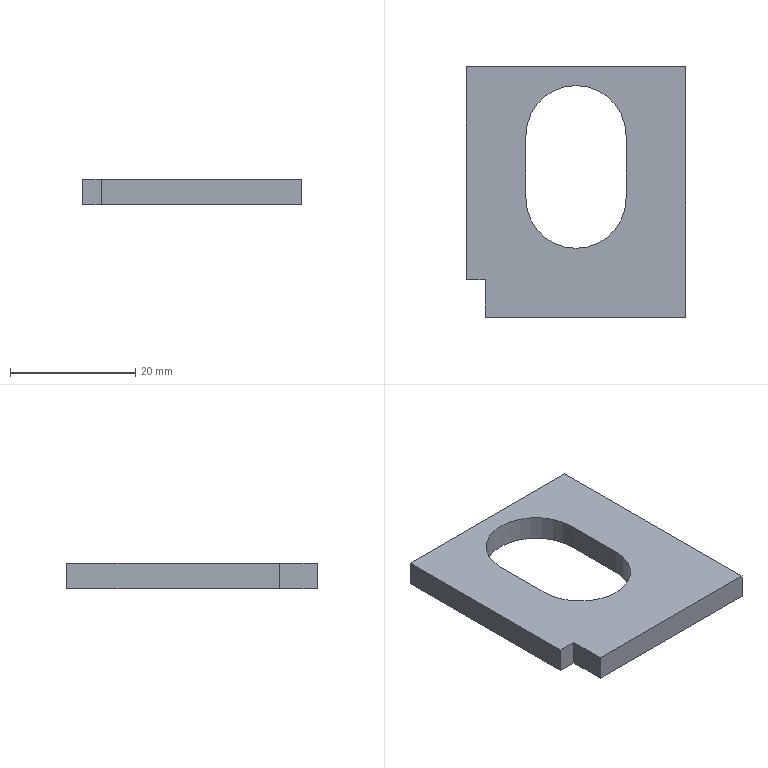Part | SolidWorks | features Extrusion 1 | 1 solid | 12 faces | box 35 x 40 x 4 mm | volume 4084 mm3 | plane 10 | cylinder 2 | commonest cylinder face diameters 16 x2
STEP:
#1=CARTESIAN_POINT('',(35.,0.,4.));
#2=VERTEX_POINT('',#1);
#3=CARTESIAN_POINT('',(35.,40.,4.));
#4=VERTEX_POINT('',#3);
#5=CARTESIAN_POINT('',(35.,0.,4.));
#6=DIRECTION('',(0.,1.,0.));
#7=VECTOR('',#6,1000.);
#8=LINE('',#5,#7);
#9=EDGE_CURVE('',#2,#4,#8,.T.);
#10=ORIENTED_EDGE('',*,*,#9,.T.);
#11=CARTESIAN_POINT('',(0.,40.,4.));
#12=VERTEX_POINT('',#11);
#13=CARTESIAN_POINT('',(0.,40.,4.));
#14=DIRECTION('',(-1.,0.,0.));
#15=VECTOR('',#14,1000.);
#16=LINE('',#13,#15);
#17=EDGE_CURVE('',#4,#12,#16,.T.);
#18=ORIENTED_EDGE('',*,*,#17,.T.);
#19=CARTESIAN_POINT('',(0.,5.998,4.));
#20=VERTEX_POINT('',#19);
#21=CARTESIAN_POINT('',(0.,5.998,4.));
#22=DIRECTION('',(0.,-1.,0.));
#23=VECTOR('',#22,1000.);
#24=LINE('',#21,#23);
#25=EDGE_CURVE('',#12,#20,#24,.T.);
#26=ORIENTED_EDGE('',*,*,#25,.T.);
#27=CARTESIAN_POINT('',(3.,5.998,4.));
#28=VERTEX_POINT('',#27);
#29=CARTESIAN_POINT('',(0.,5.998,4.));
#30=DIRECTION('',(1.,0.,0.));
#31=VECTOR('',#30,1000.);
#32=LINE('',#29,#31);
#33=EDGE_CURVE('',#20,#28,#32,.T.);
#34=ORIENTED_EDGE('',*,*,#33,.T.);
#35=CARTESIAN_POINT('',(3.,0.,4.));
#36=VERTEX_POINT('',#35);
#37=CARTESIAN_POINT('',(3.,5.998,4.));
#38=DIRECTION('',(0.,-1.,0.));
#39=VECTOR('',#38,1000.);
#40=LINE('',#37,#39);
#41=EDGE_CURVE('',#28,#36,#40,.T.);
#42=ORIENTED_EDGE('',*,*,#41,.T.);
#43=CARTESIAN_POINT('',(3.,0.,4.));
#44=DIRECTION('',(1.,0.,0.));
#45=VECTOR('',#44,1000.);
#46=LINE('',#43,#45);
#47=EDGE_CURVE('',#36,#2,#46,.T.);
#48=ORIENTED_EDGE('',*,*,#47,.T.);
#49=EDGE_LOOP('',(#10,#18,#26,#34,#42,#48));
#50=FACE_OUTER_BOUND('',#49,.T.);
#51=CARTESIAN_POINT('',(25.5,29.,4.));
#52=VERTEX_POINT('',#51);
#53=CARTESIAN_POINT('',(9.5,29.,4.));
#54=VERTEX_POINT('',#53);
#55=CARTESIAN_POINT('',(17.5,29.,4.));
#56=DIRECTION('',(0.,0.,1.));
#57=DIRECTION('',(1.,0.,0.));
#58=AXIS2_PLACEMENT_3D('',#55,#56,#57);
#59=CIRCLE('',#58,8.);
#60=EDGE_CURVE('',#52,#54,#59,.T.);
#61=ORIENTED_EDGE('',*,*,#60,.F.);
#62=CARTESIAN_POINT('',(25.5,19.,4.));
#63=VERTEX_POINT('',#62);
#64=CARTESIAN_POINT('',(25.5,29.,4.));
#65=DIRECTION('',(0.,1.,0.));
#66=VECTOR('',#65,1000.);
#67=LINE('',#64,#66);
#68=EDGE_CURVE('',#63,#52,#67,.T.);
#69=ORIENTED_EDGE('',*,*,#68,.F.);
#70=CARTESIAN_POINT('',(9.5,19.,4.));
#71=VERTEX_POINT('',#70);
#72=CARTESIAN_POINT('',(17.5,19.,4.));
#73=DIRECTION('',(0.,0.,1.));
#74=DIRECTION('',(1.,0.,0.));
#75=AXIS2_PLACEMENT_3D('',#72,#73,#74);
#76=CIRCLE('',#75,8.);
#77=EDGE_CURVE('',#71,#63,#76,.T.);
#78=ORIENTED_EDGE('',*,*,#77,.F.);
#79=CARTESIAN_POINT('',(9.5,29.,4.));
#80=DIRECTION('',(0.,-1.,0.));
#81=VECTOR('',#80,1000.);
#82=LINE('',#79,#81);
#83=EDGE_CURVE('',#54,#71,#82,.T.);
#84=ORIENTED_EDGE('',*,*,#83,.F.);
#85=EDGE_LOOP('',(#61,#69,#78,#84));
#86=FACE_BOUND('',#85,.T.);
#87=CARTESIAN_POINT('',(0.,0.,4.));
#88=DIRECTION('',(0.,0.,-1.));
#89=DIRECTION('',(-1.,0.,0.));
#90=AXIS2_PLACEMENT_3D('',#87,#88,#89);
#91=PLANE('',#90);
#92=ADVANCED_FACE('',(#50,#86),#91,.F.);
#93=CARTESIAN_POINT('',(35.,0.,0.));
#94=VERTEX_POINT('',#93);
#95=CARTESIAN_POINT('',(35.,40.,0.));
#96=VERTEX_POINT('',#95);
#97=CARTESIAN_POINT('',(35.,0.,0.));
#98=DIRECTION('',(0.,1.,0.));
#99=VECTOR('',#98,1000.);
#100=LINE('',#97,#99);
#101=EDGE_CURVE('',#94,#96,#100,.T.);
#102=ORIENTED_EDGE('',*,*,#101,.F.);
#103=CARTESIAN_POINT('',(3.,0.,0.));
#104=VERTEX_POINT('',#103);
#105=CARTESIAN_POINT('',(3.,0.,0.));
#106=DIRECTION('',(1.,0.,0.));
#107=VECTOR('',#106,1000.);
#108=LINE('',#105,#107);
#109=EDGE_CURVE('',#104,#94,#108,.T.);
#110=ORIENTED_EDGE('',*,*,#109,.F.);
#111=CARTESIAN_POINT('',(3.,5.998,0.));
#112=VERTEX_POINT('',#111);
#113=CARTESIAN_POINT('',(3.,5.998,0.));
#114=DIRECTION('',(0.,-1.,0.));
#115=VECTOR('',#114,1000.);
#116=LINE('',#113,#115);
#117=EDGE_CURVE('',#112,#104,#116,.T.);
#118=ORIENTED_EDGE('',*,*,#117,.F.);
#119=CARTESIAN_POINT('',(0.,5.998,0.));
#120=VERTEX_POINT('',#119);
#121=CARTESIAN_POINT('',(0.,5.998,0.));
#122=DIRECTION('',(1.,0.,0.));
#123=VECTOR('',#122,1000.);
#124=LINE('',#121,#123);
#125=EDGE_CURVE('',#120,#112,#124,.T.);
#126=ORIENTED_EDGE('',*,*,#125,.F.);
#127=CARTESIAN_POINT('',(0.,40.,0.));
#128=VERTEX_POINT('',#127);
#129=CARTESIAN_POINT('',(0.,5.998,0.));
#130=DIRECTION('',(0.,-1.,0.));
#131=VECTOR('',#130,1000.);
#132=LINE('',#129,#131);
#133=EDGE_CURVE('',#128,#120,#132,.T.);
#134=ORIENTED_EDGE('',*,*,#133,.F.);
#135=CARTESIAN_POINT('',(0.,40.,0.));
#136=DIRECTION('',(-1.,0.,0.));
#137=VECTOR('',#136,1000.);
#138=LINE('',#135,#137);
#139=EDGE_CURVE('',#96,#128,#138,.T.);
#140=ORIENTED_EDGE('',*,*,#139,.F.);
#141=EDGE_LOOP('',(#102,#110,#118,#126,#134,#140));
#142=FACE_OUTER_BOUND('',#141,.T.);
#143=CARTESIAN_POINT('',(25.5,19.,0.));
#144=VERTEX_POINT('',#143);
#145=CARTESIAN_POINT('',(25.5,29.,0.));
#146=VERTEX_POINT('',#145);
#147=CARTESIAN_POINT('',(25.5,29.,0.));
#148=DIRECTION('',(0.,1.,0.));
#149=VECTOR('',#148,1000.);
#150=LINE('',#147,#149);
#151=EDGE_CURVE('',#144,#146,#150,.T.);
#152=ORIENTED_EDGE('',*,*,#151,.T.);
#153=CARTESIAN_POINT('',(9.5,29.,0.));
#154=VERTEX_POINT('',#153);
#155=CARTESIAN_POINT('',(17.5,29.,0.));
#156=DIRECTION('',(0.,0.,1.));
#157=DIRECTION('',(1.,0.,0.));
#158=AXIS2_PLACEMENT_3D('',#155,#156,#157);
#159=CIRCLE('',#158,8.);
#160=EDGE_CURVE('',#146,#154,#159,.T.);
#161=ORIENTED_EDGE('',*,*,#160,.T.);
#162=CARTESIAN_POINT('',(9.5,19.,0.));
#163=VERTEX_POINT('',#162);
#164=CARTESIAN_POINT('',(9.5,29.,0.));
#165=DIRECTION('',(0.,-1.,0.));
#166=VECTOR('',#165,1000.);
#167=LINE('',#164,#166);
#168=EDGE_CURVE('',#154,#163,#167,.T.);
#169=ORIENTED_EDGE('',*,*,#168,.T.);
#170=CARTESIAN_POINT('',(17.5,19.,0.));
#171=DIRECTION('',(0.,0.,1.));
#172=DIRECTION('',(1.,0.,0.));
#173=AXIS2_PLACEMENT_3D('',#170,#171,#172);
#174=CIRCLE('',#173,8.);
#175=EDGE_CURVE('',#163,#144,#174,.T.);
#176=ORIENTED_EDGE('',*,*,#175,.T.);
#177=EDGE_LOOP('',(#152,#161,#169,#176));
#178=FACE_BOUND('',#177,.T.);
#179=CARTESIAN_POINT('',(0.,0.,0.));
#180=DIRECTION('',(0.,0.,-1.));
#181=DIRECTION('',(-1.,0.,0.));
#182=AXIS2_PLACEMENT_3D('',#179,#180,#181);
#183=PLANE('',#182);
#184=ADVANCED_FACE('',(#142,#178),#183,.T.);
#185=ORIENTED_EDGE('',*,*,#101,.T.);
#186=CARTESIAN_POINT('',(35.,40.,4.));
#187=DIRECTION('',(0.,0.,-1.));
#188=VECTOR('',#187,1000.);
#189=LINE('',#186,#188);
#190=EDGE_CURVE('',#4,#96,#189,.T.);
#191=ORIENTED_EDGE('',*,*,#190,.F.);
#192=ORIENTED_EDGE('',*,*,#9,.F.);
#193=CARTESIAN_POINT('',(35.,0.,4.));
#194=DIRECTION('',(0.,0.,-1.));
#195=VECTOR('',#194,1000.);
#196=LINE('',#193,#195);
#197=EDGE_CURVE('',#2,#94,#196,.T.);
#198=ORIENTED_EDGE('',*,*,#197,.T.);
#199=EDGE_LOOP('',(#185,#191,#192,#198));
#200=FACE_OUTER_BOUND('',#199,.T.);
#201=CARTESIAN_POINT('',(35.,0.,4.));
#202=DIRECTION('',(-1.,0.,0.));
#203=DIRECTION('',(0.,0.,1.));
#204=AXIS2_PLACEMENT_3D('',#201,#202,#203);
#205=PLANE('',#204);
#206=ADVANCED_FACE('',(#200),#205,.F.);
#207=ORIENTED_EDGE('',*,*,#139,.T.);
#208=CARTESIAN_POINT('',(0.,40.,4.));
#209=DIRECTION('',(0.,0.,-1.));
#210=VECTOR('',#209,1000.);
#211=LINE('',#208,#210);
#212=EDGE_CURVE('',#12,#128,#211,.T.);
#213=ORIENTED_EDGE('',*,*,#212,.F.);
#214=ORIENTED_EDGE('',*,*,#17,.F.);
#215=ORIENTED_EDGE('',*,*,#190,.T.);
#216=EDGE_LOOP('',(#207,#213,#214,#215));
#217=FACE_OUTER_BOUND('',#216,.T.);
#218=CARTESIAN_POINT('',(0.,40.,4.));
#219=DIRECTION('',(0.,-1.,0.));
#220=DIRECTION('',(0.,0.,-1.));
#221=AXIS2_PLACEMENT_3D('',#218,#219,#220);
#222=PLANE('',#221);
#223=ADVANCED_FACE('',(#217),#222,.F.);
#224=ORIENTED_EDGE('',*,*,#133,.T.);
#225=CARTESIAN_POINT('',(0.,5.998,4.));
#226=DIRECTION('',(0.,0.,-1.));
#227=VECTOR('',#226,1000.);
#228=LINE('',#225,#227);
#229=EDGE_CURVE('',#20,#120,#228,.T.);
#230=ORIENTED_EDGE('',*,*,#229,.F.);
#231=ORIENTED_EDGE('',*,*,#25,.F.);
#232=ORIENTED_EDGE('',*,*,#212,.T.);
#233=EDGE_LOOP('',(#224,#230,#231,#232));
#234=FACE_OUTER_BOUND('',#233,.T.);
#235=CARTESIAN_POINT('',(0.,5.998,4.));
#236=DIRECTION('',(1.,0.,0.));
#237=DIRECTION('',(0.,0.,-1.));
#238=AXIS2_PLACEMENT_3D('',#235,#236,#237);
#239=PLANE('',#238);
#240=ADVANCED_FACE('',(#234),#239,.F.);
#241=ORIENTED_EDGE('',*,*,#125,.T.);
#242=CARTESIAN_POINT('',(3.,5.998,4.));
#243=DIRECTION('',(0.,0.,-1.));
#244=VECTOR('',#243,1000.);
#245=LINE('',#242,#244);
#246=EDGE_CURVE('',#28,#112,#245,.T.);
#247=ORIENTED_EDGE('',*,*,#246,.F.);
#248=ORIENTED_EDGE('',*,*,#33,.F.);
#249=ORIENTED_EDGE('',*,*,#229,.T.);
#250=EDGE_LOOP('',(#241,#247,#248,#249));
#251=FACE_OUTER_BOUND('',#250,.T.);
#252=CARTESIAN_POINT('',(0.,5.998,4.));
#253=DIRECTION('',(0.,1.,0.));
#254=DIRECTION('',(0.,0.,1.));
#255=AXIS2_PLACEMENT_3D('',#252,#253,#254);
#256=PLANE('',#255);
#257=ADVANCED_FACE('',(#251),#256,.F.);
#258=ORIENTED_EDGE('',*,*,#117,.T.);
#259=CARTESIAN_POINT('',(3.,0.,4.));
#260=DIRECTION('',(0.,0.,-1.));
#261=VECTOR('',#260,1000.);
#262=LINE('',#259,#261);
#263=EDGE_CURVE('',#36,#104,#262,.T.);
#264=ORIENTED_EDGE('',*,*,#263,.F.);
#265=ORIENTED_EDGE('',*,*,#41,.F.);
#266=ORIENTED_EDGE('',*,*,#246,.T.);
#267=EDGE_LOOP('',(#258,#264,#265,#266));
#268=FACE_OUTER_BOUND('',#267,.T.);
#269=CARTESIAN_POINT('',(3.,5.998,4.));
#270=DIRECTION('',(1.,0.,0.));
#271=DIRECTION('',(0.,0.,-1.));
#272=AXIS2_PLACEMENT_3D('',#269,#270,#271);
#273=PLANE('',#272);
#274=ADVANCED_FACE('',(#268),#273,.F.);
#275=ORIENTED_EDGE('',*,*,#109,.T.);
#276=ORIENTED_EDGE('',*,*,#197,.F.);
#277=ORIENTED_EDGE('',*,*,#47,.F.);
#278=ORIENTED_EDGE('',*,*,#263,.T.);
#279=EDGE_LOOP('',(#275,#276,#277,#278));
#280=FACE_OUTER_BOUND('',#279,.T.);
#281=CARTESIAN_POINT('',(3.,0.,4.));
#282=DIRECTION('',(0.,1.,0.));
#283=DIRECTION('',(0.,0.,1.));
#284=AXIS2_PLACEMENT_3D('',#281,#282,#283);
#285=PLANE('',#284);
#286=ADVANCED_FACE('',(#280),#285,.F.);
#287=ORIENTED_EDGE('',*,*,#160,.F.);
#288=CARTESIAN_POINT('',(25.5,29.,4.));
#289=DIRECTION('',(0.,0.,-1.));
#290=VECTOR('',#289,1000.);
#291=LINE('',#288,#290);
#292=EDGE_CURVE('',#52,#146,#291,.T.);
#293=ORIENTED_EDGE('',*,*,#292,.F.);
#294=ORIENTED_EDGE('',*,*,#60,.T.);
#295=CARTESIAN_POINT('',(9.5,29.,4.));
#296=DIRECTION('',(0.,0.,-1.));
#297=VECTOR('',#296,1000.);
#298=LINE('',#295,#297);
#299=EDGE_CURVE('',#54,#154,#298,.T.);
#300=ORIENTED_EDGE('',*,*,#299,.T.);
#301=EDGE_LOOP('',(#287,#293,#294,#300));
#302=FACE_OUTER_BOUND('',#301,.T.);
#303=CARTESIAN_POINT('',(17.5,29.,4.));
#304=DIRECTION('',(0.,0.,-1.));
#305=DIRECTION('',(-1.,0.,0.));
#306=AXIS2_PLACEMENT_3D('',#303,#304,#305);
#307=CYLINDRICAL_SURFACE('',#306,8.);
#308=ADVANCED_FACE('',(#302),#307,.F.);
#309=ORIENTED_EDGE('',*,*,#168,.F.);
#310=ORIENTED_EDGE('',*,*,#299,.F.);
#311=ORIENTED_EDGE('',*,*,#83,.T.);
#312=CARTESIAN_POINT('',(9.5,19.,4.));
#313=DIRECTION('',(0.,0.,-1.));
#314=VECTOR('',#313,1000.);
#315=LINE('',#312,#314);
#316=EDGE_CURVE('',#71,#163,#315,.T.);
#317=ORIENTED_EDGE('',*,*,#316,.T.);
#318=EDGE_LOOP('',(#309,#310,#311,#317));
#319=FACE_OUTER_BOUND('',#318,.T.);
#320=CARTESIAN_POINT('',(9.5,29.,4.));
#321=DIRECTION('',(1.,0.,0.));
#322=DIRECTION('',(0.,0.,-1.));
#323=AXIS2_PLACEMENT_3D('',#320,#321,#322);
#324=PLANE('',#323);
#325=ADVANCED_FACE('',(#319),#324,.T.);
#326=ORIENTED_EDGE('',*,*,#175,.F.);
#327=ORIENTED_EDGE('',*,*,#316,.F.);
#328=ORIENTED_EDGE('',*,*,#77,.T.);
#329=CARTESIAN_POINT('',(25.5,19.,4.));
#330=DIRECTION('',(0.,0.,-1.));
#331=VECTOR('',#330,1000.);
#332=LINE('',#329,#331);
#333=EDGE_CURVE('',#63,#144,#332,.T.);
#334=ORIENTED_EDGE('',*,*,#333,.T.);
#335=EDGE_LOOP('',(#326,#327,#328,#334));
#336=FACE_OUTER_BOUND('',#335,.T.);
#337=CARTESIAN_POINT('',(17.5,19.,4.));
#338=DIRECTION('',(0.,0.,-1.));
#339=DIRECTION('',(-1.,0.,0.));
#340=AXIS2_PLACEMENT_3D('',#337,#338,#339);
#341=CYLINDRICAL_SURFACE('',#340,8.);
#342=ADVANCED_FACE('',(#336),#341,.F.);
#343=ORIENTED_EDGE('',*,*,#151,.F.);
#344=ORIENTED_EDGE('',*,*,#333,.F.);
#345=ORIENTED_EDGE('',*,*,#68,.T.);
#346=ORIENTED_EDGE('',*,*,#292,.T.);
#347=EDGE_LOOP('',(#343,#344,#345,#346));
#348=FACE_OUTER_BOUND('',#347,.T.);
#349=CARTESIAN_POINT('',(25.5,29.,4.));
#350=DIRECTION('',(-1.,0.,0.));
#351=DIRECTION('',(0.,0.,1.));
#352=AXIS2_PLACEMENT_3D('',#349,#350,#351);
#353=PLANE('',#352);
#354=ADVANCED_FACE('',(#348),#353,.T.);
#355=CLOSED_SHELL('',(#92,#184,#206,#223,#240,#257,#274,#286,#308,#325,#342,#354));
#356=MANIFOLD_SOLID_BREP('',#355);
#357=CARTESIAN_POINT('',(0.,0.,0.));
#358=DIRECTION('',(0.,0.,1.));
#359=DIRECTION('',(1.,0.,0.));
#360=AXIS2_PLACEMENT_3D('',#357,#358,#359);
#361=(LENGTH_UNIT()NAMED_UNIT(*)SI_UNIT(.MILLI.,.METRE.));
#362=UNCERTAINTY_MEASURE_WITH_UNIT(LENGTH_MEASURE(0.00001),#361,'','');
#363=(NAMED_UNIT(*)PLANE_ANGLE_UNIT()SI_UNIT($,.RADIAN.));
#364=(NAMED_UNIT(*)SI_UNIT($,.STERADIAN.)SOLID_ANGLE_UNIT());
#365=(GEOMETRIC_REPRESENTATION_CONTEXT(3)GLOBAL_UNCERTAINTY_ASSIGNED_CONTEXT((#362))GLOBAL_UNIT_ASSIGNED_CONTEXT((#361,#363,#364))REPRESENTATION_CONTEXT('',''));
#366=ADVANCED_BREP_SHAPE_REPRESENTATION('',(#356,#360),#365);